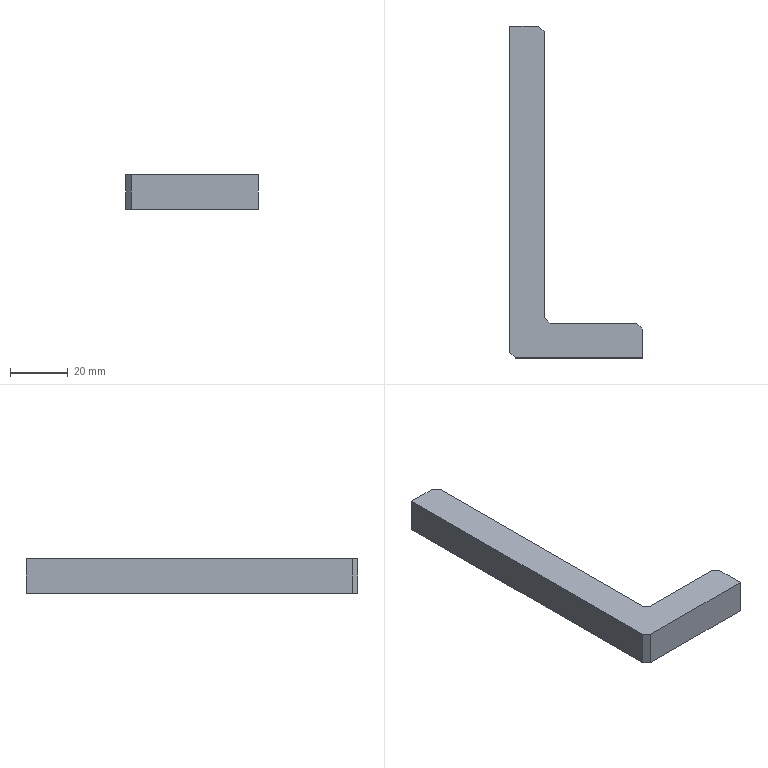Part | SolidWorks | features Chamfer 3, Extrusion 1 | 1 solid | 12 faces | box 46 x 115 x 12 mm | volume 21408 mm3 | plane 12
STEP:
#1=CARTESIAN_POINT('',(2.,0.,6.));
#2=VERTEX_POINT('',#1);
#3=CARTESIAN_POINT('',(46.,0.,6.));
#4=VERTEX_POINT('',#3);
#5=CARTESIAN_POINT('',(46.,0.,6.));
#6=DIRECTION('',(1.,0.,0.));
#7=VECTOR('',#6,1000.);
#8=LINE('',#5,#7);
#9=EDGE_CURVE('',#2,#4,#8,.T.);
#10=ORIENTED_EDGE('',*,*,#9,.F.);
#11=CARTESIAN_POINT('',(2.,0.,-6.));
#12=VERTEX_POINT('',#11);
#13=CARTESIAN_POINT('',(2.,0.,6.));
#14=DIRECTION('',(0.,0.,-1.));
#15=VECTOR('',#14,1000.);
#16=LINE('',#13,#15);
#17=EDGE_CURVE('',#2,#12,#16,.T.);
#18=ORIENTED_EDGE('',*,*,#17,.T.);
#19=CARTESIAN_POINT('',(46.,0.,-6.));
#20=VERTEX_POINT('',#19);
#21=CARTESIAN_POINT('',(46.,0.,-6.));
#22=DIRECTION('',(1.,0.,0.));
#23=VECTOR('',#22,1000.);
#24=LINE('',#21,#23);
#25=EDGE_CURVE('',#12,#20,#24,.T.);
#26=ORIENTED_EDGE('',*,*,#25,.T.);
#27=CARTESIAN_POINT('',(46.,0.,6.));
#28=DIRECTION('',(0.,0.,-1.));
#29=VECTOR('',#28,1000.);
#30=LINE('',#27,#29);
#31=EDGE_CURVE('',#4,#20,#30,.T.);
#32=ORIENTED_EDGE('',*,*,#31,.F.);
#33=EDGE_LOOP('',(#10,#18,#26,#32));
#34=FACE_OUTER_BOUND('',#33,.T.);
#35=CARTESIAN_POINT('',(46.,0.,6.));
#36=DIRECTION('',(0.,1.,0.));
#37=DIRECTION('',(-1.,0.,0.));
#38=AXIS2_PLACEMENT_3D('',#35,#36,#37);
#39=PLANE('',#38);
#40=ADVANCED_FACE('',(#34),#39,.F.);
#41=CARTESIAN_POINT('',(46.,10.,-6.));
#42=VERTEX_POINT('',#41);
#43=CARTESIAN_POINT('',(46.,12.,-6.));
#44=DIRECTION('',(0.,1.,0.));
#45=VECTOR('',#44,1000.);
#46=LINE('',#43,#45);
#47=EDGE_CURVE('',#20,#42,#46,.T.);
#48=ORIENTED_EDGE('',*,*,#47,.T.);
#49=CARTESIAN_POINT('',(46.,10.,6.));
#50=VERTEX_POINT('',#49);
#51=CARTESIAN_POINT('',(46.,10.,6.));
#52=DIRECTION('',(0.,0.,1.));
#53=VECTOR('',#52,1000.);
#54=LINE('',#51,#53);
#55=EDGE_CURVE('',#42,#50,#54,.T.);
#56=ORIENTED_EDGE('',*,*,#55,.T.);
#57=CARTESIAN_POINT('',(46.,12.,6.));
#58=DIRECTION('',(0.,1.,0.));
#59=VECTOR('',#58,1000.);
#60=LINE('',#57,#59);
#61=EDGE_CURVE('',#4,#50,#60,.T.);
#62=ORIENTED_EDGE('',*,*,#61,.F.);
#63=ORIENTED_EDGE('',*,*,#31,.T.);
#64=EDGE_LOOP('',(#48,#56,#62,#63));
#65=FACE_OUTER_BOUND('',#64,.T.);
#66=CARTESIAN_POINT('',(46.,12.,6.));
#67=DIRECTION('',(-1.,0.,0.));
#68=DIRECTION('',(0.,0.,1.));
#69=AXIS2_PLACEMENT_3D('',#66,#67,#68);
#70=PLANE('',#69);
#71=ADVANCED_FACE('',(#65),#70,.F.);
#72=CARTESIAN_POINT('',(44.,12.,6.));
#73=VERTEX_POINT('',#72);
#74=CARTESIAN_POINT('',(14.,12.,6.));
#75=VERTEX_POINT('',#74);
#76=CARTESIAN_POINT('',(12.,12.,6.));
#77=DIRECTION('',(-1.,0.,0.));
#78=VECTOR('',#77,1000.);
#79=LINE('',#76,#78);
#80=EDGE_CURVE('',#73,#75,#79,.T.);
#81=ORIENTED_EDGE('',*,*,#80,.F.);
#82=CARTESIAN_POINT('',(44.,12.,-6.));
#83=VERTEX_POINT('',#82);
#84=CARTESIAN_POINT('',(44.,12.,6.));
#85=DIRECTION('',(0.,0.,-1.));
#86=VECTOR('',#85,1000.);
#87=LINE('',#84,#86);
#88=EDGE_CURVE('',#73,#83,#87,.T.);
#89=ORIENTED_EDGE('',*,*,#88,.T.);
#90=CARTESIAN_POINT('',(14.,12.,-6.));
#91=VERTEX_POINT('',#90);
#92=CARTESIAN_POINT('',(12.,12.,-6.));
#93=DIRECTION('',(-1.,0.,0.));
#94=VECTOR('',#93,1000.);
#95=LINE('',#92,#94);
#96=EDGE_CURVE('',#83,#91,#95,.T.);
#97=ORIENTED_EDGE('',*,*,#96,.T.);
#98=CARTESIAN_POINT('',(14.,12.,6.));
#99=DIRECTION('',(0.,0.,1.));
#100=VECTOR('',#99,1000.);
#101=LINE('',#98,#100);
#102=EDGE_CURVE('',#91,#75,#101,.T.);
#103=ORIENTED_EDGE('',*,*,#102,.T.);
#104=EDGE_LOOP('',(#81,#89,#97,#103));
#105=FACE_OUTER_BOUND('',#104,.T.);
#106=CARTESIAN_POINT('',(12.,12.,6.));
#107=DIRECTION('',(0.,-1.,0.));
#108=DIRECTION('',(0.,0.,-1.));
#109=AXIS2_PLACEMENT_3D('',#106,#107,#108);
#110=PLANE('',#109);
#111=ADVANCED_FACE('',(#105),#110,.F.);
#112=CARTESIAN_POINT('',(12.,14.,-6.));
#113=VERTEX_POINT('',#112);
#114=CARTESIAN_POINT('',(12.,113.,-6.));
#115=VERTEX_POINT('',#114);
#116=CARTESIAN_POINT('',(12.,115.,-6.));
#117=DIRECTION('',(0.,1.,0.));
#118=VECTOR('',#117,1000.);
#119=LINE('',#116,#118);
#120=EDGE_CURVE('',#113,#115,#119,.T.);
#121=ORIENTED_EDGE('',*,*,#120,.T.);
#122=CARTESIAN_POINT('',(12.,113.,6.));
#123=VERTEX_POINT('',#122);
#124=CARTESIAN_POINT('',(12.,113.,6.));
#125=DIRECTION('',(0.,0.,1.));
#126=VECTOR('',#125,1000.);
#127=LINE('',#124,#126);
#128=EDGE_CURVE('',#115,#123,#127,.T.);
#129=ORIENTED_EDGE('',*,*,#128,.T.);
#130=CARTESIAN_POINT('',(12.,14.,6.));
#131=VERTEX_POINT('',#130);
#132=CARTESIAN_POINT('',(12.,115.,6.));
#133=DIRECTION('',(0.,1.,0.));
#134=VECTOR('',#133,1000.);
#135=LINE('',#132,#134);
#136=EDGE_CURVE('',#131,#123,#135,.T.);
#137=ORIENTED_EDGE('',*,*,#136,.F.);
#138=CARTESIAN_POINT('',(12.,14.,-6.));
#139=DIRECTION('',(0.,0.,-1.));
#140=VECTOR('',#139,1000.);
#141=LINE('',#138,#140);
#142=EDGE_CURVE('',#131,#113,#141,.T.);
#143=ORIENTED_EDGE('',*,*,#142,.T.);
#144=EDGE_LOOP('',(#121,#129,#137,#143));
#145=FACE_OUTER_BOUND('',#144,.T.);
#146=CARTESIAN_POINT('',(12.,115.,6.));
#147=DIRECTION('',(-1.,0.,0.));
#148=DIRECTION('',(0.,-1.,0.));
#149=AXIS2_PLACEMENT_3D('',#146,#147,#148);
#150=PLANE('',#149);
#151=ADVANCED_FACE('',(#145),#150,.F.);
#152=CARTESIAN_POINT('',(10.,115.,6.));
#153=VERTEX_POINT('',#152);
#154=CARTESIAN_POINT('',(0.,115.,6.));
#155=VERTEX_POINT('',#154);
#156=CARTESIAN_POINT('',(0.,115.,6.));
#157=DIRECTION('',(-1.,0.,0.));
#158=VECTOR('',#157,1000.);
#159=LINE('',#156,#158);
#160=EDGE_CURVE('',#153,#155,#159,.T.);
#161=ORIENTED_EDGE('',*,*,#160,.F.);
#162=CARTESIAN_POINT('',(10.,115.,-6.));
#163=VERTEX_POINT('',#162);
#164=CARTESIAN_POINT('',(10.,115.,6.));
#165=DIRECTION('',(0.,0.,-1.));
#166=VECTOR('',#165,1000.);
#167=LINE('',#164,#166);
#168=EDGE_CURVE('',#153,#163,#167,.T.);
#169=ORIENTED_EDGE('',*,*,#168,.T.);
#170=CARTESIAN_POINT('',(0.,115.,-6.));
#171=VERTEX_POINT('',#170);
#172=CARTESIAN_POINT('',(0.,115.,-6.));
#173=DIRECTION('',(-1.,0.,0.));
#174=VECTOR('',#173,1000.);
#175=LINE('',#172,#174);
#176=EDGE_CURVE('',#163,#171,#175,.T.);
#177=ORIENTED_EDGE('',*,*,#176,.T.);
#178=CARTESIAN_POINT('',(0.,115.,6.));
#179=DIRECTION('',(0.,0.,-1.));
#180=VECTOR('',#179,1000.);
#181=LINE('',#178,#180);
#182=EDGE_CURVE('',#155,#171,#181,.T.);
#183=ORIENTED_EDGE('',*,*,#182,.F.);
#184=EDGE_LOOP('',(#161,#169,#177,#183));
#185=FACE_OUTER_BOUND('',#184,.T.);
#186=CARTESIAN_POINT('',(0.,115.,6.));
#187=DIRECTION('',(0.,-1.,0.));
#188=DIRECTION('',(0.,0.,-1.));
#189=AXIS2_PLACEMENT_3D('',#186,#187,#188);
#190=PLANE('',#189);
#191=ADVANCED_FACE('',(#185),#190,.F.);
#192=CARTESIAN_POINT('',(0.,2.,-6.));
#193=VERTEX_POINT('',#192);
#194=CARTESIAN_POINT('',(0.,0.,-6.));
#195=DIRECTION('',(0.,-1.,0.));
#196=VECTOR('',#195,1000.);
#197=LINE('',#194,#196);
#198=EDGE_CURVE('',#171,#193,#197,.T.);
#199=ORIENTED_EDGE('',*,*,#198,.T.);
#200=CARTESIAN_POINT('',(0.,2.,6.));
#201=VERTEX_POINT('',#200);
#202=CARTESIAN_POINT('',(0.,2.,6.));
#203=DIRECTION('',(0.,0.,1.));
#204=VECTOR('',#203,1000.);
#205=LINE('',#202,#204);
#206=EDGE_CURVE('',#193,#201,#205,.T.);
#207=ORIENTED_EDGE('',*,*,#206,.T.);
#208=CARTESIAN_POINT('',(0.,0.,6.));
#209=DIRECTION('',(0.,-1.,0.));
#210=VECTOR('',#209,1000.);
#211=LINE('',#208,#210);
#212=EDGE_CURVE('',#155,#201,#211,.T.);
#213=ORIENTED_EDGE('',*,*,#212,.F.);
#214=ORIENTED_EDGE('',*,*,#182,.T.);
#215=EDGE_LOOP('',(#199,#207,#213,#214));
#216=FACE_OUTER_BOUND('',#215,.T.);
#217=CARTESIAN_POINT('',(0.,0.,6.));
#218=DIRECTION('',(1.,0.,0.));
#219=DIRECTION('',(0.,0.,-1.));
#220=AXIS2_PLACEMENT_3D('',#217,#218,#219);
#221=PLANE('',#220);
#222=ADVANCED_FACE('',(#216),#221,.F.);
#223=ORIENTED_EDGE('',*,*,#61,.T.);
#224=CARTESIAN_POINT('',(44.,12.,6.));
#225=DIRECTION('',(-0.7071,0.7071,0.));
#226=VECTOR('',#225,1000.);
#227=LINE('',#224,#226);
#228=EDGE_CURVE('',#50,#73,#227,.T.);
#229=ORIENTED_EDGE('',*,*,#228,.T.);
#230=ORIENTED_EDGE('',*,*,#80,.T.);
#231=CARTESIAN_POINT('',(13.,13.,6.));
#232=DIRECTION('',(-0.7071,0.7071,0.));
#233=VECTOR('',#232,1000.);
#234=LINE('',#231,#233);
#235=EDGE_CURVE('',#75,#131,#234,.T.);
#236=ORIENTED_EDGE('',*,*,#235,.T.);
#237=ORIENTED_EDGE('',*,*,#136,.T.);
#238=CARTESIAN_POINT('',(10.,115.,6.));
#239=DIRECTION('',(-0.7071,0.7071,0.));
#240=VECTOR('',#239,1000.);
#241=LINE('',#238,#240);
#242=EDGE_CURVE('',#123,#153,#241,.T.);
#243=ORIENTED_EDGE('',*,*,#242,.T.);
#244=ORIENTED_EDGE('',*,*,#160,.T.);
#245=ORIENTED_EDGE('',*,*,#212,.T.);
#246=CARTESIAN_POINT('',(2.,0.,6.));
#247=DIRECTION('',(0.7071,-0.7071,0.));
#248=VECTOR('',#247,1000.);
#249=LINE('',#246,#248);
#250=EDGE_CURVE('',#201,#2,#249,.T.);
#251=ORIENTED_EDGE('',*,*,#250,.T.);
#252=ORIENTED_EDGE('',*,*,#9,.T.);
#253=EDGE_LOOP('',(#223,#229,#230,#236,#237,#243,#244,#245,#251,#252));
#254=FACE_OUTER_BOUND('',#253,.T.);
#255=CARTESIAN_POINT('',(0.,0.,6.));
#256=DIRECTION('',(0.,0.,-1.));
#257=DIRECTION('',(-1.,0.,0.));
#258=AXIS2_PLACEMENT_3D('',#255,#256,#257);
#259=PLANE('',#258);
#260=ADVANCED_FACE('',(#254),#259,.F.);
#261=ORIENTED_EDGE('',*,*,#96,.F.);
#262=CARTESIAN_POINT('',(28.,28.,-6.));
#263=DIRECTION('',(0.7071,-0.7071,0.));
#264=VECTOR('',#263,1000.);
#265=LINE('',#262,#264);
#266=EDGE_CURVE('',#83,#42,#265,.T.);
#267=ORIENTED_EDGE('',*,*,#266,.T.);
#268=ORIENTED_EDGE('',*,*,#47,.F.);
#269=ORIENTED_EDGE('',*,*,#25,.F.);
#270=CARTESIAN_POINT('',(1.,1.,-6.));
#271=DIRECTION('',(-0.7071,0.7071,0.));
#272=VECTOR('',#271,1000.);
#273=LINE('',#270,#272);
#274=EDGE_CURVE('',#12,#193,#273,.T.);
#275=ORIENTED_EDGE('',*,*,#274,.T.);
#276=ORIENTED_EDGE('',*,*,#198,.F.);
#277=ORIENTED_EDGE('',*,*,#176,.F.);
#278=CARTESIAN_POINT('',(62.5,62.5,-6.));
#279=DIRECTION('',(0.7071,-0.7071,0.));
#280=VECTOR('',#279,1000.);
#281=LINE('',#278,#280);
#282=EDGE_CURVE('',#163,#115,#281,.T.);
#283=ORIENTED_EDGE('',*,*,#282,.T.);
#284=ORIENTED_EDGE('',*,*,#120,.F.);
#285=CARTESIAN_POINT('',(12.,14.,-6.));
#286=DIRECTION('',(0.7071,-0.7071,0.));
#287=VECTOR('',#286,1000.);
#288=LINE('',#285,#287);
#289=EDGE_CURVE('',#113,#91,#288,.T.);
#290=ORIENTED_EDGE('',*,*,#289,.T.);
#291=EDGE_LOOP('',(#261,#267,#268,#269,#275,#276,#277,#283,#284,#290));
#292=FACE_OUTER_BOUND('',#291,.T.);
#293=CARTESIAN_POINT('',(0.,0.,-6.));
#294=DIRECTION('',(0.,0.,-1.));
#295=DIRECTION('',(-1.,0.,0.));
#296=AXIS2_PLACEMENT_3D('',#293,#294,#295);
#297=PLANE('',#296);
#298=ADVANCED_FACE('',(#292),#297,.T.);
#299=ORIENTED_EDGE('',*,*,#235,.F.);
#300=ORIENTED_EDGE('',*,*,#102,.F.);
#301=ORIENTED_EDGE('',*,*,#289,.F.);
#302=ORIENTED_EDGE('',*,*,#142,.F.);
#303=EDGE_LOOP('',(#299,#300,#301,#302));
#304=FACE_OUTER_BOUND('',#303,.T.);
#305=CARTESIAN_POINT('',(12.,14.,6.));
#306=DIRECTION('',(0.7071,0.7071,0.));
#307=DIRECTION('',(0.,0.,1.));
#308=AXIS2_PLACEMENT_3D('',#305,#306,#307);
#309=PLANE('',#308);
#310=ADVANCED_FACE('',(#304),#309,.T.);
#311=ORIENTED_EDGE('',*,*,#250,.F.);
#312=ORIENTED_EDGE('',*,*,#206,.F.);
#313=ORIENTED_EDGE('',*,*,#274,.F.);
#314=ORIENTED_EDGE('',*,*,#17,.F.);
#315=EDGE_LOOP('',(#311,#312,#313,#314));
#316=FACE_OUTER_BOUND('',#315,.T.);
#317=CARTESIAN_POINT('',(2.,0.,6.));
#318=DIRECTION('',(0.7071,0.7071,0.));
#319=DIRECTION('',(0.,0.,-1.));
#320=AXIS2_PLACEMENT_3D('',#317,#318,#319);
#321=PLANE('',#320);
#322=ADVANCED_FACE('',(#316),#321,.F.);
#323=ORIENTED_EDGE('',*,*,#228,.F.);
#324=ORIENTED_EDGE('',*,*,#55,.F.);
#325=ORIENTED_EDGE('',*,*,#266,.F.);
#326=ORIENTED_EDGE('',*,*,#88,.F.);
#327=EDGE_LOOP('',(#323,#324,#325,#326));
#328=FACE_OUTER_BOUND('',#327,.T.);
#329=CARTESIAN_POINT('',(44.,12.,6.));
#330=DIRECTION('',(-0.7071,-0.7071,0.));
#331=DIRECTION('',(0.,0.,-1.));
#332=AXIS2_PLACEMENT_3D('',#329,#330,#331);
#333=PLANE('',#332);
#334=ADVANCED_FACE('',(#328),#333,.F.);
#335=ORIENTED_EDGE('',*,*,#242,.F.);
#336=ORIENTED_EDGE('',*,*,#128,.F.);
#337=ORIENTED_EDGE('',*,*,#282,.F.);
#338=ORIENTED_EDGE('',*,*,#168,.F.);
#339=EDGE_LOOP('',(#335,#336,#337,#338));
#340=FACE_OUTER_BOUND('',#339,.T.);
#341=CARTESIAN_POINT('',(10.,115.,6.));
#342=DIRECTION('',(-0.7071,-0.7071,0.));
#343=DIRECTION('',(0.,0.,-1.));
#344=AXIS2_PLACEMENT_3D('',#341,#342,#343);
#345=PLANE('',#344);
#346=ADVANCED_FACE('',(#340),#345,.F.);
#347=CLOSED_SHELL('',(#40,#71,#111,#151,#191,#222,#260,#298,#310,#322,#334,#346));
#348=MANIFOLD_SOLID_BREP('',#347);
#349=CARTESIAN_POINT('',(0.,0.,0.));
#350=DIRECTION('',(0.,0.,1.));
#351=DIRECTION('',(1.,0.,0.));
#352=AXIS2_PLACEMENT_3D('',#349,#350,#351);
#353=(LENGTH_UNIT()NAMED_UNIT(*)SI_UNIT(.MILLI.,.METRE.));
#354=UNCERTAINTY_MEASURE_WITH_UNIT(LENGTH_MEASURE(0.00001),#353,'','');
#355=(NAMED_UNIT(*)PLANE_ANGLE_UNIT()SI_UNIT($,.RADIAN.));
#356=(NAMED_UNIT(*)SI_UNIT($,.STERADIAN.)SOLID_ANGLE_UNIT());
#357=(GEOMETRIC_REPRESENTATION_CONTEXT(3)GLOBAL_UNCERTAINTY_ASSIGNED_CONTEXT((#354))GLOBAL_UNIT_ASSIGNED_CONTEXT((#353,#355,#356))REPRESENTATION_CONTEXT('',''));
#358=ADVANCED_BREP_SHAPE_REPRESENTATION('',(#348,#352),#357);